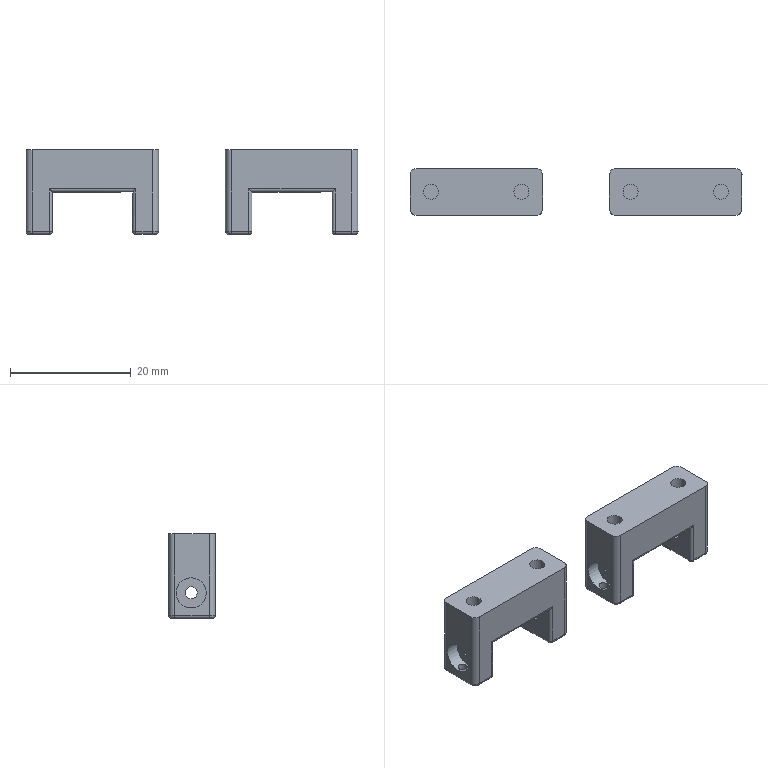Part | 2 solids | 94 faces | box 54.928 x 7.717 x 14 mm | volume 2964 mm3 | cylinder 52 | plane 28 | torus 8 | sphere 6 | commonest cylinder face diameters 1 x28 2 x12 1.6 x4 2.5 x4 5 x4